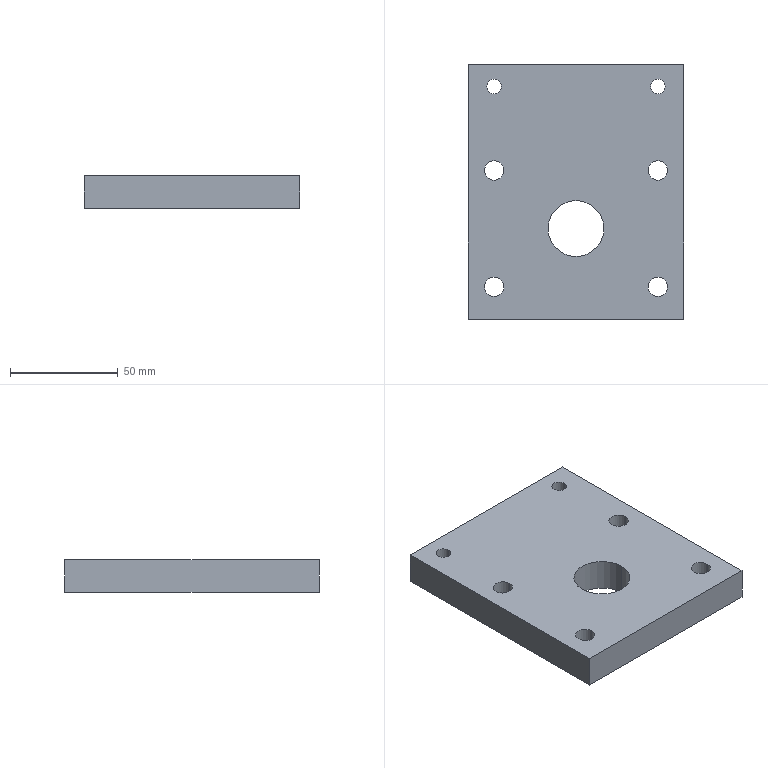Part | STEP file | 0244_219_Plate | 1 solid | 20 faces | box 100 x 118 x 15 mm | volume 164130 mm3 | cylinder 14 | plane 6 | commonest cylinder face diameters 9 x8 6.8 x4 26 x2